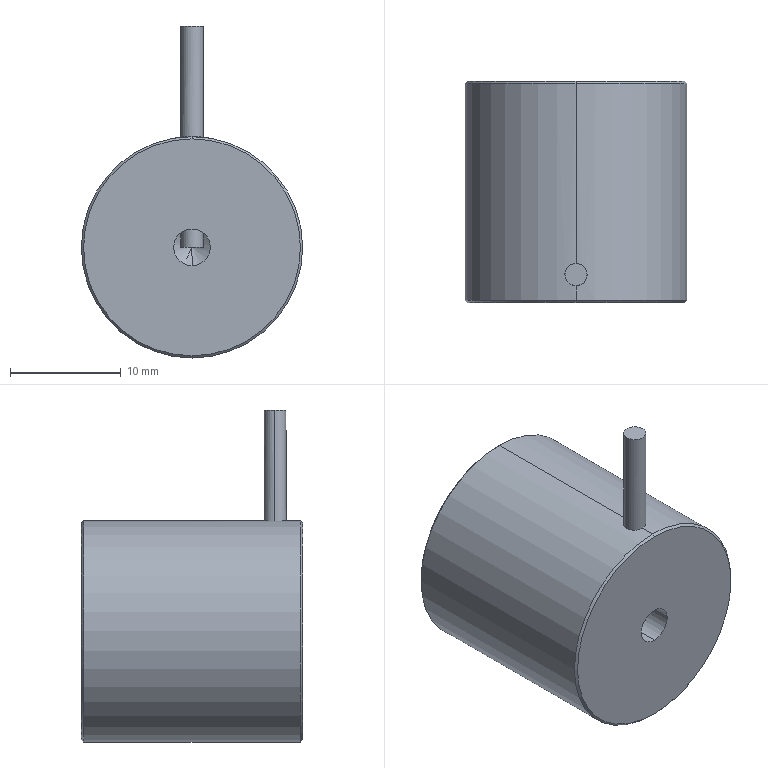Part | SolidWorks | features BaseBody 1 | 1 solid | 18 faces | box 20 x 20 x 30 mm | volume 6254 mm3 | cylinder 8 | cone 6 | plane 4 | commonest cylinder face diameters 2 x4 3.3 x2 20 x2
STEP:
#1=CARTESIAN_POINT('',(0.,20.,9.8));
#2=VERTEX_POINT('',#1);
#3=CARTESIAN_POINT('',(0.,19.8,10.));
#4=VERTEX_POINT('',#3);
#5=CARTESIAN_POINT('',(0.,20.,9.8));
#6=DIRECTION('',(0.,-0.7071,0.7071));
#7=VECTOR('',#6,1000.);
#8=LINE('',#5,#7);
#9=EDGE_CURVE('',#2,#4,#8,.T.);
#10=ORIENTED_EDGE('',*,*,#9,.F.);
#11=CARTESIAN_POINT('',(0.,20.,-9.8));
#12=VERTEX_POINT('',#11);
#13=CARTESIAN_POINT('',(0.,20.,0.));
#14=DIRECTION('',(0.,1.,0.));
#15=DIRECTION('',(0.,0.,1.));
#16=AXIS2_PLACEMENT_3D('',#13,#14,#15);
#17=CIRCLE('',#16,9.8);
#18=EDGE_CURVE('',#12,#2,#17,.T.);
#19=ORIENTED_EDGE('',*,*,#18,.F.);
#20=CARTESIAN_POINT('',(0.,19.8,-10.));
#21=VERTEX_POINT('',#20);
#22=CARTESIAN_POINT('',(0.,20.,-9.8));
#23=DIRECTION('',(0.,-0.7071,-0.7071));
#24=VECTOR('',#23,1000.);
#25=LINE('',#22,#24);
#26=EDGE_CURVE('',#12,#21,#25,.T.);
#27=ORIENTED_EDGE('',*,*,#26,.T.);
#28=CARTESIAN_POINT('',(0.,19.8,0.));
#29=DIRECTION('',(0.,-1.,0.));
#30=DIRECTION('',(0.,0.,1.));
#31=AXIS2_PLACEMENT_3D('',#28,#29,#30);
#32=CIRCLE('',#31,10.);
#33=EDGE_CURVE('',#4,#21,#32,.T.);
#34=ORIENTED_EDGE('',*,*,#33,.F.);
#35=EDGE_LOOP('',(#10,#19,#27,#34));
#36=FACE_OUTER_BOUND('',#35,.T.);
#37=CARTESIAN_POINT('',(0.,20.,0.));
#38=DIRECTION('',(0.,-1.,0.));
#39=DIRECTION('',(0.,0.,-1.));
#40=AXIS2_PLACEMENT_3D('',#37,#38,#39);
#41=CONICAL_SURFACE('',#40,9.8,0.7854);
#42=ADVANCED_FACE('',(#36),#41,.T.);
#43=CARTESIAN_POINT('',(0.,0.,-9.8));
#44=VERTEX_POINT('',#43);
#45=CARTESIAN_POINT('',(0.,0.2,-10.));
#46=VERTEX_POINT('',#45);
#47=CARTESIAN_POINT('',(0.,0.2,-10.));
#48=DIRECTION('',(0.,0.7071,-0.7071));
#49=VECTOR('',#48,1000.);
#50=LINE('',#47,#49);
#51=EDGE_CURVE('',#44,#46,#50,.T.);
#52=ORIENTED_EDGE('',*,*,#51,.F.);
#53=CARTESIAN_POINT('',(0.,0.,9.8));
#54=VERTEX_POINT('',#53);
#55=CARTESIAN_POINT('',(0.,0.,0.));
#56=DIRECTION('',(0.,-1.,0.));
#57=DIRECTION('',(0.,0.,1.));
#58=AXIS2_PLACEMENT_3D('',#55,#56,#57);
#59=CIRCLE('',#58,9.8);
#60=EDGE_CURVE('',#54,#44,#59,.T.);
#61=ORIENTED_EDGE('',*,*,#60,.F.);
#62=CARTESIAN_POINT('',(0.,0.2,10.));
#63=VERTEX_POINT('',#62);
#64=CARTESIAN_POINT('',(0.,0.2,10.));
#65=DIRECTION('',(0.,0.7071,0.7071));
#66=VECTOR('',#65,1000.);
#67=LINE('',#64,#66);
#68=EDGE_CURVE('',#54,#63,#67,.T.);
#69=ORIENTED_EDGE('',*,*,#68,.T.);
#70=CARTESIAN_POINT('',(0.,0.2,0.));
#71=DIRECTION('',(0.,1.,0.));
#72=DIRECTION('',(0.,0.,1.));
#73=AXIS2_PLACEMENT_3D('',#70,#71,#72);
#74=CIRCLE('',#73,10.);
#75=EDGE_CURVE('',#46,#63,#74,.T.);
#76=ORIENTED_EDGE('',*,*,#75,.F.);
#77=EDGE_LOOP('',(#52,#61,#69,#76));
#78=FACE_OUTER_BOUND('',#77,.T.);
#79=CARTESIAN_POINT('',(0.,0.2,0.));
#80=DIRECTION('',(0.,1.,0.));
#81=DIRECTION('',(0.,0.,1.));
#82=AXIS2_PLACEMENT_3D('',#79,#80,#81);
#83=CONICAL_SURFACE('',#82,10.,0.7854);
#84=ADVANCED_FACE('',(#78),#83,.T.);
#85=CARTESIAN_POINT('',(-1.,2.5,20.));
#86=VERTEX_POINT('',#85);
#87=CARTESIAN_POINT('',(1.,2.5,20.));
#88=VERTEX_POINT('',#87);
#89=CARTESIAN_POINT('',(0.,2.5,20.));
#90=DIRECTION('',(0.,0.,1.));
#91=DIRECTION('',(1.,0.,0.));
#92=AXIS2_PLACEMENT_3D('',#89,#90,#91);
#93=CIRCLE('',#92,1.);
#94=EDGE_CURVE('',#86,#88,#93,.T.);
#95=ORIENTED_EDGE('',*,*,#94,.T.);
#96=CARTESIAN_POINT('',(0.,2.5,20.));
#97=DIRECTION('',(0.,0.,1.));
#98=DIRECTION('',(1.,0.,0.));
#99=AXIS2_PLACEMENT_3D('',#96,#97,#98);
#100=CIRCLE('',#99,1.);
#101=EDGE_CURVE('',#88,#86,#100,.T.);
#102=ORIENTED_EDGE('',*,*,#101,.T.);
#103=EDGE_LOOP('',(#95,#102));
#104=FACE_OUTER_BOUND('',#103,.T.);
#105=CARTESIAN_POINT('',(0.,2.5,20.));
#106=DIRECTION('',(0.,0.,1.));
#107=DIRECTION('',(1.,0.,0.));
#108=AXIS2_PLACEMENT_3D('',#105,#106,#107);
#109=PLANE('',#108);
#110=ADVANCED_FACE('',(#104),#109,.T.);
#111=CARTESIAN_POINT('',(1.,2.5,9.95));
#112=VERTEX_POINT('',#111);
#113=CARTESIAN_POINT('',(1.,2.5,20.));
#114=DIRECTION('',(0.,0.,-1.));
#115=VECTOR('',#114,1000.);
#116=LINE('',#113,#115);
#117=EDGE_CURVE('',#88,#112,#116,.T.);
#118=ORIENTED_EDGE('',*,*,#117,.F.);
#119=ORIENTED_EDGE('',*,*,#94,.F.);
#120=CARTESIAN_POINT('',(-1.,2.5,9.95));
#121=VERTEX_POINT('',#120);
#122=CARTESIAN_POINT('',(-1.,2.5,20.));
#123=DIRECTION('',(0.,0.,-1.));
#124=VECTOR('',#123,1000.);
#125=LINE('',#122,#124);
#126=EDGE_CURVE('',#86,#121,#125,.T.);
#127=ORIENTED_EDGE('',*,*,#126,.T.);
#128=CARTESIAN_POINT('',(0.,1.5,10.));
#129=VERTEX_POINT('',#128);
#130=CARTESIAN_POINT('',(-1.,2.5,9.95));
#131=CARTESIAN_POINT('',(-1.,2.438,9.95));
#132=CARTESIAN_POINT('',(-0.9942,2.374,9.95));
#133=CARTESIAN_POINT('',(-0.9756,2.278,9.952));
#134=CARTESIAN_POINT('',(-0.9677,2.246,9.953));
#135=CARTESIAN_POINT('',(-0.9532,2.197,9.954));
#136=CARTESIAN_POINT('',(-0.9453,2.173,9.955));
#137=CARTESIAN_POINT('',(-0.9349,2.145,9.956));
#138=CARTESIAN_POINT('',(-0.9302,2.133,9.957));
#139=CARTESIAN_POINT('',(-0.927,2.125,9.957));
#140=CARTESIAN_POINT('',(-0.9247,2.119,9.957));
#141=CARTESIAN_POINT('',(-0.9067,2.076,9.959));
#142=CARTESIAN_POINT('',(-0.883,2.026,9.961));
#143=CARTESIAN_POINT('',(-0.8138,1.915,9.967));
#144=CARTESIAN_POINT('',(-0.7677,1.853,9.971));
#145=CARTESIAN_POINT('',(-0.646,1.732,9.979));
#146=CARTESIAN_POINT('',(-0.5848,1.686,9.983));
#147=CARTESIAN_POINT('',(-0.5016,1.634,9.987));
#148=CARTESIAN_POINT('',(-0.4752,1.62,9.989));
#149=CARTESIAN_POINT('',(-0.4384,1.601,9.99));
#150=CARTESIAN_POINT('',(-0.4206,1.593,9.991));
#151=CARTESIAN_POINT('',(-0.4012,1.584,9.992));
#152=CARTESIAN_POINT('',(-0.3931,1.581,9.992));
#153=CARTESIAN_POINT('',(-0.3878,1.578,9.992));
#154=CARTESIAN_POINT('',(-0.3866,1.578,9.993));
#155=CARTESIAN_POINT('',(-0.2552,1.523,9.998));
#156=CARTESIAN_POINT('',(-0.1238,1.5,10.));
#157=CARTESIAN_POINT('',(0.,1.5,10.));
#158=B_SPLINE_CURVE_WITH_KNOTS('',3,(#130,#131,#132,#133,#134,#135,#136,#137,#138,#139,#140,#141,#142,#143,#144,#145,#146,#147,#148,#149,#150,#151,#152,#153,#154,#155,#156,#157),.UNSPECIFIED.,.F.,.F.,(4,2,2,1,1,2,2,2,2,2,2,1,1,2,2,4),(0.,0.125,0.1875,0.2188,0.2344,0.2422,0.25,0.375,0.5,0.625,0.6875,0.7188,0.7344,0.7422,0.75,1.),.UNSPECIFIED.);
#159=EDGE_CURVE('',#121,#129,#158,.T.);
#160=ORIENTED_EDGE('',*,*,#159,.T.);
#161=CARTESIAN_POINT('',(0.,1.5,10.));
#162=CARTESIAN_POINT('',(0.06188,1.5,10.));
#163=CARTESIAN_POINT('',(0.1256,1.506,9.999));
#164=CARTESIAN_POINT('',(0.222,1.524,9.998));
#165=CARTESIAN_POINT('',(0.2542,1.532,9.997));
#166=CARTESIAN_POINT('',(0.3025,1.547,9.995));
#167=CARTESIAN_POINT('',(0.3267,1.555,9.995));
#168=CARTESIAN_POINT('',(0.3547,1.565,9.994));
#169=CARTESIAN_POINT('',(0.3667,1.57,9.993));
#170=CARTESIAN_POINT('',(0.3747,1.573,9.993));
#171=CARTESIAN_POINT('',(0.3801,1.575,9.993));
#172=CARTESIAN_POINT('',(0.4653,1.61,9.99));
#173=CARTESIAN_POINT('',(0.5848,1.671,9.984));
#174=CARTESIAN_POINT('',(0.7683,1.854,9.971));
#175=CARTESIAN_POINT('',(0.814,1.915,9.967));
#176=CARTESIAN_POINT('',(0.8659,1.999,9.963));
#177=CARTESIAN_POINT('',(0.8805,2.025,9.961));
#178=CARTESIAN_POINT('',(0.899,2.062,9.96));
#179=CARTESIAN_POINT('',(0.9075,2.08,9.959));
#180=CARTESIAN_POINT('',(0.9161,2.099,9.958));
#181=CARTESIAN_POINT('',(0.9195,2.107,9.958));
#182=CARTESIAN_POINT('',(0.9217,2.112,9.957));
#183=CARTESIAN_POINT('',(0.9222,2.113,9.957));
#184=CARTESIAN_POINT('',(0.9767,2.245,9.952));
#185=CARTESIAN_POINT('',(1.,2.376,9.95));
#186=CARTESIAN_POINT('',(1.,2.5,9.95));
#187=B_SPLINE_CURVE_WITH_KNOTS('',3,(#161,#162,#163,#164,#165,#166,#167,#168,#169,#170,#171,#172,#173,#174,#175,#176,#177,#178,#179,#180,#181,#182,#183,#184,#185,#186),.UNSPECIFIED.,.F.,.F.,(4,2,2,1,1,2,2,2,2,2,1,1,2,2,4),(0.,0.125,0.1875,0.2187,0.2344,0.2422,0.25,0.5,0.625,0.6875,0.7188,0.7344,0.7422,0.75,1.),.UNSPECIFIED.);
#188=EDGE_CURVE('',#129,#112,#187,.T.);
#189=ORIENTED_EDGE('',*,*,#188,.T.);
#190=EDGE_LOOP('',(#118,#119,#127,#160,#189));
#191=FACE_OUTER_BOUND('',#190,.T.);
#192=CARTESIAN_POINT('',(0.,2.5,20.));
#193=DIRECTION('',(0.,0.,-1.));
#194=DIRECTION('',(-1.,0.,0.));
#195=AXIS2_PLACEMENT_3D('',#192,#193,#194);
#196=CYLINDRICAL_SURFACE('',#195,1.);
#197=ADVANCED_FACE('',(#191),#196,.T.);
#198=CARTESIAN_POINT('',(1.,2.5,1.312));
#199=VERTEX_POINT('',#198);
#200=CARTESIAN_POINT('',(1.,2.5,0.));
#201=VERTEX_POINT('',#200);
#202=CARTESIAN_POINT('',(1.,2.5,20.));
#203=DIRECTION('',(0.,0.,-1.));
#204=VECTOR('',#203,1000.);
#205=LINE('',#202,#204);
#206=EDGE_CURVE('',#199,#201,#205,.T.);
#207=ORIENTED_EDGE('',*,*,#206,.F.);
#208=CARTESIAN_POINT('',(0.,1.5,1.65));
#209=VERTEX_POINT('',#208);
#210=CARTESIAN_POINT('',(1.,2.5,1.312));
#211=CARTESIAN_POINT('',(1.,2.439,1.312));
#212=CARTESIAN_POINT('',(0.9944,2.375,1.317));
#213=CARTESIAN_POINT('',(0.9754,2.277,1.331));
#214=CARTESIAN_POINT('',(0.9673,2.244,1.337));
#215=CARTESIAN_POINT('',(0.9523,2.194,1.348));
#216=CARTESIAN_POINT('',(0.944,2.169,1.353));
#217=CARTESIAN_POINT('',(0.9347,2.145,1.36));
#218=CARTESIAN_POINT('',(0.9283,2.128,1.364));
#219=CARTESIAN_POINT('',(0.9241,2.118,1.367));
#220=CARTESIAN_POINT('',(0.9105,2.086,1.376));
#221=CARTESIAN_POINT('',(0.8978,2.058,1.385));
#222=CARTESIAN_POINT('',(0.875,2.016,1.399));
#223=CARTESIAN_POINT('',(0.8628,1.994,1.407));
#224=CARTESIAN_POINT('',(0.8467,1.968,1.416));
#225=CARTESIAN_POINT('',(0.8383,1.955,1.421));
#226=CARTESIAN_POINT('',(0.8345,1.949,1.423));
#227=CARTESIAN_POINT('',(0.832,1.945,1.425));
#228=CARTESIAN_POINT('',(0.8297,1.942,1.426));
#229=CARTESIAN_POINT('',(0.8265,1.937,1.428));
#230=CARTESIAN_POINT('',(0.8162,1.921,1.434));
#231=CARTESIAN_POINT('',(0.7872,1.883,1.45));
#232=CARTESIAN_POINT('',(0.7753,1.868,1.457));
#233=CARTESIAN_POINT('',(0.7533,1.842,1.468));
#234=CARTESIAN_POINT('',(0.7412,1.829,1.474));
#235=CARTESIAN_POINT('',(0.7252,1.811,1.482));
#236=CARTESIAN_POINT('',(0.7179,1.804,1.486));
#237=CARTESIAN_POINT('',(0.713,1.799,1.488));
#238=CARTESIAN_POINT('',(0.7096,1.795,1.49));
#239=CARTESIAN_POINT('',(0.6521,1.738,1.517));
#240=CARTESIAN_POINT('',(0.5949,1.694,1.54));
#241=CARTESIAN_POINT('',(0.5136,1.641,1.568));
#242=CARTESIAN_POINT('',(0.4872,1.626,1.576));
#243=CARTESIAN_POINT('',(0.4492,1.606,1.588));
#244=CARTESIAN_POINT('',(0.4306,1.597,1.593));
#245=CARTESIAN_POINT('',(0.4097,1.588,1.598));
#246=CARTESIAN_POINT('',(0.4009,1.584,1.601));
#247=CARTESIAN_POINT('',(0.395,1.581,1.602));
#248=CARTESIAN_POINT('',(0.3933,1.581,1.602));
#249=CARTESIAN_POINT('',(0.2614,1.525,1.634));
#250=CARTESIAN_POINT('',(0.1277,1.5,1.65));
#251=CARTESIAN_POINT('',(0.,1.5,1.65));
#252=B_SPLINE_CURVE_WITH_KNOTS('',3,(#210,#211,#212,#213,#214,#215,#216,#217,#218,#219,#220,#221,#222,#223,#224,#225,#226,#227,#228,#229,#230,#231,#232,#233,#234,#235,#236,#237,#238,#239,#240,#241,#242,#243,#244,#245,#246,#247,#248,#249,#250,#251),.UNSPECIFIED.,.F.,.F.,(4,2,2,1,2,2,2,1,1,1,2,2,2,2,1,1,2,2,2,2,1,1,2,2,4),(0.,0.125,0.1875,0.2188,0.2344,0.25,0.3125,0.3438,0.3594,0.3672,0.3711,0.375,0.4375,0.4688,0.4844,0.4922,0.4961,0.5,0.625,0.6875,0.7188,0.7344,0.7422,0.75,1.),.UNSPECIFIED.);
#253=EDGE_CURVE('',#199,#209,#252,.T.);
#254=ORIENTED_EDGE('',*,*,#253,.T.);
#255=CARTESIAN_POINT('',(-1.,2.5,1.312));
#256=VERTEX_POINT('',#255);
#257=CARTESIAN_POINT('',(0.,1.5,1.65));
#258=CARTESIAN_POINT('',(-0.06387,1.5,1.65));
#259=CARTESIAN_POINT('',(-0.1292,1.506,1.646));
#260=CARTESIAN_POINT('',(-0.2272,1.526,1.634));
#261=CARTESIAN_POINT('',(-0.26,1.534,1.63));
#262=CARTESIAN_POINT('',(-0.3088,1.549,1.621));
#263=CARTESIAN_POINT('',(-0.3331,1.557,1.616));
#264=CARTESIAN_POINT('',(-0.3613,1.567,1.61));
#265=CARTESIAN_POINT('',(-0.3734,1.572,1.607));
#266=CARTESIAN_POINT('',(-0.3814,1.576,1.605));
#267=CARTESIAN_POINT('',(-0.3865,1.578,1.604));
#268=CARTESIAN_POINT('',(-0.4353,1.598,1.592));
#269=CARTESIAN_POINT('',(-0.4867,1.624,1.577));
#270=CARTESIAN_POINT('',(-0.5681,1.676,1.549));
#271=CARTESIAN_POINT('',(-0.5959,1.696,1.539));
#272=CARTESIAN_POINT('',(-0.638,1.73,1.522));
#273=CARTESIAN_POINT('',(-0.6592,1.748,1.513));
#274=CARTESIAN_POINT('',(-0.6838,1.77,1.502));
#275=CARTESIAN_POINT('',(-0.6961,1.782,1.496));
#276=CARTESIAN_POINT('',(-0.7013,1.787,1.494));
#277=CARTESIAN_POINT('',(-0.7048,1.791,1.492));
#278=CARTESIAN_POINT('',(-0.7058,1.792,1.491));
#279=CARTESIAN_POINT('',(-0.7495,1.835,1.471));
#280=CARTESIAN_POINT('',(-0.7778,1.871,1.456));
#281=CARTESIAN_POINT('',(-0.8067,1.909,1.44));
#282=CARTESIAN_POINT('',(-0.814,1.919,1.435));
#283=CARTESIAN_POINT('',(-0.822,1.93,1.431));
#284=CARTESIAN_POINT('',(-0.8252,1.935,1.429));
#285=CARTESIAN_POINT('',(-0.8277,1.939,1.427));
#286=CARTESIAN_POINT('',(-0.8286,1.94,1.427));
#287=CARTESIAN_POINT('',(-0.829,1.941,1.427));
#288=CARTESIAN_POINT('',(-0.8282,1.94,1.427));
#289=CARTESIAN_POINT('',(-0.8497,1.972,1.415));
#290=CARTESIAN_POINT('',(-0.8672,2.001,1.404));
#291=CARTESIAN_POINT('',(-0.8899,2.044,1.389));
#292=CARTESIAN_POINT('',(-0.9004,2.065,1.383));
#293=CARTESIAN_POINT('',(-0.9097,2.085,1.377));
#294=CARTESIAN_POINT('',(-0.9156,2.098,1.373));
#295=CARTESIAN_POINT('',(-0.9177,2.103,1.371));
#296=CARTESIAN_POINT('',(-0.9771,2.243,1.331));
#297=CARTESIAN_POINT('',(-1.,2.377,1.312));
#298=CARTESIAN_POINT('',(-1.,2.5,1.312));
#299=B_SPLINE_CURVE_WITH_KNOTS('',3,(#257,#258,#259,#260,#261,#262,#263,#264,#265,#266,#267,#268,#269,#270,#271,#272,#273,#274,#275,#276,#277,#278,#279,#280,#281,#282,#283,#284,#285,#286,#287,#288,#289,#290,#291,#292,#293,#294,#295,#296,#297,#298),.UNSPECIFIED.,.F.,.F.,(4,2,2,1,1,2,2,2,2,1,1,1,2,2,2,2,1,1,2,2,2,1,2,2,4),(0.,0.125,0.1875,0.2188,0.2344,0.2422,0.25,0.375,0.4375,0.4688,0.4844,0.4922,0.4961,0.5,0.5625,0.5938,0.6094,0.6172,0.6211,0.625,0.6875,0.7188,0.7344,0.75,1.),.UNSPECIFIED.);
#300=EDGE_CURVE('',#209,#256,#299,.T.);
#301=ORIENTED_EDGE('',*,*,#300,.T.);
#302=CARTESIAN_POINT('',(-1.,2.5,0.));
#303=VERTEX_POINT('',#302);
#304=CARTESIAN_POINT('',(-1.,2.5,20.));
#305=DIRECTION('',(0.,0.,-1.));
#306=VECTOR('',#305,1000.);
#307=LINE('',#304,#306);
#308=EDGE_CURVE('',#256,#303,#307,.T.);
#309=ORIENTED_EDGE('',*,*,#308,.T.);
#310=CARTESIAN_POINT('',(0.,2.5,0.));
#311=DIRECTION('',(0.,0.,1.));
#312=DIRECTION('',(1.,0.,0.));
#313=AXIS2_PLACEMENT_3D('',#310,#311,#312);
#314=CIRCLE('',#313,1.);
#315=EDGE_CURVE('',#303,#201,#314,.T.);
#316=ORIENTED_EDGE('',*,*,#315,.T.);
#317=EDGE_LOOP('',(#207,#254,#301,#309,#316));
#318=FACE_OUTER_BOUND('',#317,.T.);
#319=CARTESIAN_POINT('',(0.,2.5,20.));
#320=DIRECTION('',(0.,0.,-1.));
#321=DIRECTION('',(-1.,0.,0.));
#322=AXIS2_PLACEMENT_3D('',#319,#320,#321);
#323=CYLINDRICAL_SURFACE('',#322,1.);
#324=ADVANCED_FACE('',(#318),#323,.T.);
#325=ORIENTED_EDGE('',*,*,#315,.F.);
#326=CARTESIAN_POINT('',(0.,2.5,0.));
#327=DIRECTION('',(0.,0.,1.));
#328=DIRECTION('',(1.,0.,0.));
#329=AXIS2_PLACEMENT_3D('',#326,#327,#328);
#330=CIRCLE('',#329,1.);
#331=EDGE_CURVE('',#201,#303,#330,.T.);
#332=ORIENTED_EDGE('',*,*,#331,.F.);
#333=EDGE_LOOP('',(#325,#332));
#334=FACE_OUTER_BOUND('',#333,.T.);
#335=CARTESIAN_POINT('',(0.,2.5,0.));
#336=DIRECTION('',(0.,0.,1.));
#337=DIRECTION('',(1.,0.,0.));
#338=AXIS2_PLACEMENT_3D('',#335,#336,#337);
#339=PLANE('',#338);
#340=ADVANCED_FACE('',(#334),#339,.F.);
#341=CARTESIAN_POINT('',(0.,8.091,0.));
#342=VERTEX_POINT('',#341);
#343=CARTESIAN_POINT('',(0.,7.1,1.65));
#344=VERTEX_POINT('',#343);
#345=CARTESIAN_POINT('',(0.,7.1,1.65));
#346=DIRECTION('',(0.,-0.515,0.8572));
#347=VECTOR('',#346,1000.);
#348=LINE('',#345,#347);
#349=EDGE_CURVE('',#342,#344,#348,.T.);
#350=ORIENTED_EDGE('',*,*,#349,.F.);
#351=CARTESIAN_POINT('',(0.,7.1,-1.65));
#352=VERTEX_POINT('',#351);
#353=CARTESIAN_POINT('',(0.,7.1,-1.65));
#354=DIRECTION('',(0.,-0.515,-0.8572));
#355=VECTOR('',#354,1000.);
#356=LINE('',#353,#355);
#357=EDGE_CURVE('',#342,#352,#356,.T.);
#358=ORIENTED_EDGE('',*,*,#357,.T.);
#359=CARTESIAN_POINT('',(0.,7.1,0.));
#360=DIRECTION('',(0.,-1.,0.));
#361=DIRECTION('',(0.,0.,-1.));
#362=AXIS2_PLACEMENT_3D('',#359,#360,#361);
#363=CIRCLE('',#362,1.65);
#364=EDGE_CURVE('',#352,#344,#363,.T.);
#365=ORIENTED_EDGE('',*,*,#364,.T.);
#366=EDGE_LOOP('',(#350,#358,#365));
#367=FACE_OUTER_BOUND('',#366,.T.);
#368=CARTESIAN_POINT('',(0.,7.1,0.));
#369=DIRECTION('',(0.,-1.,0.));
#370=DIRECTION('',(0.,0.,-1.));
#371=AXIS2_PLACEMENT_3D('',#368,#369,#370);
#372=CONICAL_SURFACE('',#371,1.65,1.03);
#373=ADVANCED_FACE('',(#367),#372,.F.);
#374=CARTESIAN_POINT('',(0.,0.,-1.65));
#375=VERTEX_POINT('',#374);
#376=CARTESIAN_POINT('',(0.,0.,1.65));
#377=VERTEX_POINT('',#376);
#378=CARTESIAN_POINT('',(0.,0.,0.));
#379=DIRECTION('',(0.,-1.,0.));
#380=DIRECTION('',(0.,0.,-1.));
#381=AXIS2_PLACEMENT_3D('',#378,#379,#380);
#382=CIRCLE('',#381,1.65);
#383=EDGE_CURVE('',#375,#377,#382,.T.);
#384=ORIENTED_EDGE('',*,*,#383,.F.);
#385=CARTESIAN_POINT('',(0.,0.,0.));
#386=DIRECTION('',(0.,-1.,0.));
#387=DIRECTION('',(0.,0.,-1.));
#388=AXIS2_PLACEMENT_3D('',#385,#386,#387);
#389=CIRCLE('',#388,1.65);
#390=EDGE_CURVE('',#377,#375,#389,.T.);
#391=ORIENTED_EDGE('',*,*,#390,.F.);
#392=EDGE_LOOP('',(#384,#391));
#393=FACE_BOUND('',#392,.T.);
#394=ORIENTED_EDGE('',*,*,#60,.T.);
#395=CARTESIAN_POINT('',(0.,0.,0.));
#396=DIRECTION('',(0.,-1.,0.));
#397=DIRECTION('',(0.,0.,1.));
#398=AXIS2_PLACEMENT_3D('',#395,#396,#397);
#399=CIRCLE('',#398,9.8);
#400=EDGE_CURVE('',#44,#54,#399,.T.);
#401=ORIENTED_EDGE('',*,*,#400,.T.);
#402=EDGE_LOOP('',(#394,#401));
#403=FACE_OUTER_BOUND('',#402,.T.);
#404=CARTESIAN_POINT('',(0.,0.,0.));
#405=DIRECTION('',(0.,1.,0.));
#406=DIRECTION('',(1.,0.,0.));
#407=AXIS2_PLACEMENT_3D('',#404,#405,#406);
#408=PLANE('',#407);
#409=ADVANCED_FACE('',(#393,#403),#408,.F.);
#410=ORIENTED_EDGE('',*,*,#18,.T.);
#411=CARTESIAN_POINT('',(0.,20.,0.));
#412=DIRECTION('',(0.,1.,0.));
#413=DIRECTION('',(0.,0.,1.));
#414=AXIS2_PLACEMENT_3D('',#411,#412,#413);
#415=CIRCLE('',#414,9.8);
#416=EDGE_CURVE('',#2,#12,#415,.T.);
#417=ORIENTED_EDGE('',*,*,#416,.T.);
#418=EDGE_LOOP('',(#410,#417));
#419=FACE_OUTER_BOUND('',#418,.T.);
#420=CARTESIAN_POINT('',(0.,20.,0.));
#421=DIRECTION('',(0.,1.,0.));
#422=DIRECTION('',(1.,0.,0.));
#423=AXIS2_PLACEMENT_3D('',#420,#421,#422);
#424=PLANE('',#423);
#425=ADVANCED_FACE('',(#419),#424,.T.);
#426=CARTESIAN_POINT('',(0.,3.5,1.65));
#427=VERTEX_POINT('',#426);
#428=CARTESIAN_POINT('',(0.,0.,1.65));
#429=DIRECTION('',(0.,-1.,0.));
#430=VECTOR('',#429,1000.);
#431=LINE('',#428,#430);
#432=EDGE_CURVE('',#344,#427,#431,.T.);
#433=ORIENTED_EDGE('',*,*,#432,.F.);
#434=ORIENTED_EDGE('',*,*,#364,.F.);
#435=CARTESIAN_POINT('',(0.,0.,-1.65));
#436=DIRECTION('',(0.,-1.,0.));
#437=VECTOR('',#436,1000.);
#438=LINE('',#435,#437);
#439=EDGE_CURVE('',#352,#375,#438,.T.);
#440=ORIENTED_EDGE('',*,*,#439,.T.);
#441=ORIENTED_EDGE('',*,*,#383,.T.);
#442=CARTESIAN_POINT('',(0.,0.,1.65));
#443=DIRECTION('',(0.,-1.,0.));
#444=VECTOR('',#443,1000.);
#445=LINE('',#442,#444);
#446=EDGE_CURVE('',#209,#377,#445,.T.);
#447=ORIENTED_EDGE('',*,*,#446,.F.);
#448=ORIENTED_EDGE('',*,*,#253,.F.);
#449=CARTESIAN_POINT('',(0.,3.5,1.65));
#450=CARTESIAN_POINT('',(0.06396,3.5,1.65));
#451=CARTESIAN_POINT('',(0.1293,3.494,1.646));
#452=CARTESIAN_POINT('',(0.2276,3.474,1.634));
#453=CARTESIAN_POINT('',(0.2603,3.466,1.63));
#454=CARTESIAN_POINT('',(0.3092,3.451,1.621));
#455=CARTESIAN_POINT('',(0.3336,3.443,1.616));
#456=CARTESIAN_POINT('',(0.3619,3.432,1.61));
#457=CARTESIAN_POINT('',(0.3739,3.427,1.607));
#458=CARTESIAN_POINT('',(0.382,3.424,1.605));
#459=CARTESIAN_POINT('',(0.3871,3.422,1.604));
#460=CARTESIAN_POINT('',(0.4358,3.401,1.592));
#461=CARTESIAN_POINT('',(0.4871,3.376,1.577));
#462=CARTESIAN_POINT('',(0.5685,3.323,1.549));
#463=CARTESIAN_POINT('',(0.5964,3.304,1.538));
#464=CARTESIAN_POINT('',(0.6385,3.27,1.521));
#465=CARTESIAN_POINT('',(0.6596,3.252,1.512));
#466=CARTESIAN_POINT('',(0.6843,3.229,1.501));
#467=CARTESIAN_POINT('',(0.6966,3.218,1.496));
#468=CARTESIAN_POINT('',(0.7018,3.212,1.493));
#469=CARTESIAN_POINT('',(0.7053,3.209,1.492));
#470=CARTESIAN_POINT('',(0.7063,3.208,1.491));
#471=CARTESIAN_POINT('',(0.7493,3.165,1.471));
#472=CARTESIAN_POINT('',(0.7774,3.13,1.456));
#473=CARTESIAN_POINT('',(0.8062,3.092,1.44));
#474=CARTESIAN_POINT('',(0.8137,3.081,1.436));
#475=CARTESIAN_POINT('',(0.8219,3.07,1.431));
#476=CARTESIAN_POINT('',(0.8252,3.065,1.429));
#477=CARTESIAN_POINT('',(0.828,3.061,1.427));
#478=CARTESIAN_POINT('',(0.8289,3.059,1.427));
#479=CARTESIAN_POINT('',(0.8294,3.059,1.426));
#480=CARTESIAN_POINT('',(0.8286,3.06,1.427));
#481=CARTESIAN_POINT('',(0.8502,3.028,1.414));
#482=CARTESIAN_POINT('',(0.8677,2.998,1.404));
#483=CARTESIAN_POINT('',(0.8903,2.956,1.389));
#484=CARTESIAN_POINT('',(0.9008,2.935,1.382));
#485=CARTESIAN_POINT('',(0.91,2.915,1.376));
#486=CARTESIAN_POINT('',(0.9159,2.901,1.372));
#487=CARTESIAN_POINT('',(0.9179,2.897,1.371));
#488=CARTESIAN_POINT('',(0.9772,2.756,1.331));
#489=CARTESIAN_POINT('',(1.,2.623,1.312));
#490=CARTESIAN_POINT('',(1.,2.5,1.312));
#491=B_SPLINE_CURVE_WITH_KNOTS('',3,(#449,#450,#451,#452,#453,#454,#455,#456,#457,#458,#459,#460,#461,#462,#463,#464,#465,#466,#467,#468,#469,#470,#471,#472,#473,#474,#475,#476,#477,#478,#479,#480,#481,#482,#483,#484,#485,#486,#487,#488,#489,#490),.UNSPECIFIED.,.F.,.F.,(4,2,2,1,1,2,2,2,2,1,1,1,2,2,2,2,1,1,2,2,2,1,2,2,4),(0.,0.125,0.1875,0.2188,0.2344,0.2422,0.25,0.375,0.4375,0.4688,0.4844,0.4922,0.4961,0.5,0.5625,0.5938,0.6094,0.6172,0.6211,0.625,0.6875,0.7188,0.7344,0.75,1.),.UNSPECIFIED.);
#492=EDGE_CURVE('',#427,#199,#491,.T.);
#493=ORIENTED_EDGE('',*,*,#492,.F.);
#494=EDGE_LOOP('',(#433,#434,#440,#441,#447,#448,#493));
#495=FACE_OUTER_BOUND('',#494,.T.);
#496=CARTESIAN_POINT('',(0.,0.,0.));
#497=DIRECTION('',(0.,-1.,0.));
#498=DIRECTION('',(0.,0.,-1.));
#499=AXIS2_PLACEMENT_3D('',#496,#497,#498);
#500=CYLINDRICAL_SURFACE('',#499,1.65);
#501=ADVANCED_FACE('',(#495),#500,.F.);
#502=CARTESIAN_POINT('',(0.,3.5,10.));
#503=VERTEX_POINT('',#502);
#504=CARTESIAN_POINT('',(0.,20.,10.));
#505=DIRECTION('',(0.,-1.,0.));
#506=VECTOR('',#505,1000.);
#507=LINE('',#504,#506);
#508=EDGE_CURVE('',#4,#503,#507,.T.);
#509=ORIENTED_EDGE('',*,*,#508,.F.);
#510=ORIENTED_EDGE('',*,*,#33,.T.);
#511=CARTESIAN_POINT('',(0.,20.,-10.));
#512=DIRECTION('',(0.,-1.,0.));
#513=VECTOR('',#512,1000.);
#514=LINE('',#511,#513);
#515=EDGE_CURVE('',#21,#46,#514,.T.);
#516=ORIENTED_EDGE('',*,*,#515,.T.);
#517=ORIENTED_EDGE('',*,*,#75,.T.);
#518=CARTESIAN_POINT('',(0.,20.,10.));
#519=DIRECTION('',(0.,-1.,0.));
#520=VECTOR('',#519,1000.);
#521=LINE('',#518,#520);
#522=EDGE_CURVE('',#129,#63,#521,.T.);
#523=ORIENTED_EDGE('',*,*,#522,.F.);
#524=ORIENTED_EDGE('',*,*,#159,.F.);
#525=CARTESIAN_POINT('',(0.,3.5,10.));
#526=CARTESIAN_POINT('',(-0.09534,3.5,10.));
#527=CARTESIAN_POINT('',(-0.2094,3.487,9.998));
#528=CARTESIAN_POINT('',(-0.4562,3.399,9.99));
#529=CARTESIAN_POINT('',(-0.5888,3.325,9.983));
#530=CARTESIAN_POINT('',(-0.825,3.089,9.967));
#531=CARTESIAN_POINT('',(-0.8996,2.956,9.96));
#532=CARTESIAN_POINT('',(-0.9867,2.709,9.952));
#533=CARTESIAN_POINT('',(-1.,2.595,9.95));
#534=CARTESIAN_POINT('',(-1.,2.5,9.95));
#535=B_SPLINE_CURVE_WITH_KNOTS('',3,(#525,#526,#527,#528,#529,#530,#531,#532,#533,#534),.UNSPECIFIED.,.F.,.F.,(4,2,2,2,4),(0.,0.25,0.5,0.75,1.),.UNSPECIFIED.);
#536=EDGE_CURVE('',#503,#121,#535,.T.);
#537=ORIENTED_EDGE('',*,*,#536,.F.);
#538=EDGE_LOOP('',(#509,#510,#516,#517,#523,#524,#537));
#539=FACE_OUTER_BOUND('',#538,.T.);
#540=CARTESIAN_POINT('',(0.,20.,0.));
#541=DIRECTION('',(0.,-1.,0.));
#542=DIRECTION('',(0.,0.,-1.));
#543=AXIS2_PLACEMENT_3D('',#540,#541,#542);
#544=CYLINDRICAL_SURFACE('',#543,10.);
#545=ADVANCED_FACE('',(#539),#544,.T.);
#546=CARTESIAN_POINT('',(0.,19.8,0.));
#547=DIRECTION('',(0.,-1.,0.));
#548=DIRECTION('',(0.,0.,1.));
#549=AXIS2_PLACEMENT_3D('',#546,#547,#548);
#550=CIRCLE('',#549,10.);
#551=EDGE_CURVE('',#21,#4,#550,.T.);
#552=ORIENTED_EDGE('',*,*,#551,.T.);
#553=ORIENTED_EDGE('',*,*,#508,.T.);
#554=CARTESIAN_POINT('',(1.,2.5,9.95));
#555=CARTESIAN_POINT('',(1.,2.562,9.95));
#556=CARTESIAN_POINT('',(0.9942,2.626,9.95));
#557=CARTESIAN_POINT('',(0.9756,2.722,9.952));
#558=CARTESIAN_POINT('',(0.9677,2.754,9.953));
#559=CARTESIAN_POINT('',(0.9533,2.802,9.954));
#560=CARTESIAN_POINT('',(0.9454,2.827,9.955));
#561=CARTESIAN_POINT('',(0.935,2.855,9.956));
#562=CARTESIAN_POINT('',(0.9303,2.867,9.957));
#563=CARTESIAN_POINT('',(0.9272,2.875,9.957));
#564=CARTESIAN_POINT('',(0.9249,2.88,9.957));
#565=CARTESIAN_POINT('',(0.8899,2.965,9.96));
#566=CARTESIAN_POINT('',(0.8292,3.085,9.966));
#567=CARTESIAN_POINT('',(0.6464,3.268,9.979));
#568=CARTESIAN_POINT('',(0.5852,3.313,9.983));
#569=CARTESIAN_POINT('',(0.502,3.365,9.987));
#570=CARTESIAN_POINT('',(0.4756,3.38,9.989));
#571=CARTESIAN_POINT('',(0.4388,3.399,9.99));
#572=CARTESIAN_POINT('',(0.421,3.407,9.991));
#573=CARTESIAN_POINT('',(0.4016,3.416,9.992));
#574=CARTESIAN_POINT('',(0.3936,3.419,9.992));
#575=CARTESIAN_POINT('',(0.3883,3.422,9.992));
#576=CARTESIAN_POINT('',(0.3871,3.422,9.993));
#577=CARTESIAN_POINT('',(0.2555,3.477,9.998));
#578=CARTESIAN_POINT('',(0.1239,3.5,10.));
#579=CARTESIAN_POINT('',(0.,3.5,10.));
#580=B_SPLINE_CURVE_WITH_KNOTS('',3,(#554,#555,#556,#557,#558,#559,#560,#561,#562,#563,#564,#565,#566,#567,#568,#569,#570,#571,#572,#573,#574,#575,#576,#577,#578,#579),.UNSPECIFIED.,.F.,.F.,(4,2,2,1,1,2,2,2,2,2,1,1,2,2,4),(0.,0.125,0.1875,0.2188,0.2344,0.2422,0.25,0.5,0.625,0.6875,0.7188,0.7344,0.7422,0.75,1.),.UNSPECIFIED.);
#581=EDGE_CURVE('',#112,#503,#580,.T.);
#582=ORIENTED_EDGE('',*,*,#581,.F.);
#583=ORIENTED_EDGE('',*,*,#188,.F.);
#584=ORIENTED_EDGE('',*,*,#522,.T.);
#585=CARTESIAN_POINT('',(0.,0.2,0.));
#586=DIRECTION('',(0.,1.,0.));
#587=DIRECTION('',(0.,0.,1.));
#588=AXIS2_PLACEMENT_3D('',#585,#586,#587);
#589=CIRCLE('',#588,10.);
#590=EDGE_CURVE('',#63,#46,#589,.T.);
#591=ORIENTED_EDGE('',*,*,#590,.T.);
#592=ORIENTED_EDGE('',*,*,#515,.F.);
#593=EDGE_LOOP('',(#552,#553,#582,#583,#584,#591,#592));
#594=FACE_OUTER_BOUND('',#593,.T.);
#595=CARTESIAN_POINT('',(0.,20.,0.));
#596=DIRECTION('',(0.,-1.,0.));
#597=DIRECTION('',(0.,0.,-1.));
#598=AXIS2_PLACEMENT_3D('',#595,#596,#597);
#599=CYLINDRICAL_SURFACE('',#598,10.);
#600=ADVANCED_FACE('',(#594),#599,.T.);
#601=CARTESIAN_POINT('',(0.,7.1,0.));
#602=DIRECTION('',(0.,-1.,0.));
#603=DIRECTION('',(0.,0.,-1.));
#604=AXIS2_PLACEMENT_3D('',#601,#602,#603);
#605=CIRCLE('',#604,1.65);
#606=EDGE_CURVE('',#344,#352,#605,.T.);
#607=ORIENTED_EDGE('',*,*,#606,.F.);
#608=ORIENTED_EDGE('',*,*,#432,.T.);
#609=CARTESIAN_POINT('',(-1.,2.5,1.312));
#610=CARTESIAN_POINT('',(-1.,2.561,1.312));
#611=CARTESIAN_POINT('',(-0.9944,2.625,1.317));
#612=CARTESIAN_POINT('',(-0.9754,2.723,1.331));
#613=CARTESIAN_POINT('',(-0.9673,2.756,1.337));
#614=CARTESIAN_POINT('',(-0.9523,2.806,1.348));
#615=CARTESIAN_POINT('',(-0.9441,2.831,1.353));
#616=CARTESIAN_POINT('',(-0.9347,2.855,1.36));
#617=CARTESIAN_POINT('',(-0.9283,2.872,1.364));
#618=CARTESIAN_POINT('',(-0.9241,2.882,1.367));
#619=CARTESIAN_POINT('',(-0.9106,2.914,1.376));
#620=CARTESIAN_POINT('',(-0.8978,2.942,1.385));
#621=CARTESIAN_POINT('',(-0.875,2.984,1.399));
#622=CARTESIAN_POINT('',(-0.8628,3.006,1.407));
#623=CARTESIAN_POINT('',(-0.8467,3.032,1.416));
#624=CARTESIAN_POINT('',(-0.8382,3.045,1.421));
#625=CARTESIAN_POINT('',(-0.8345,3.051,1.423));
#626=CARTESIAN_POINT('',(-0.832,3.055,1.425));
#627=CARTESIAN_POINT('',(-0.8296,3.058,1.426));
#628=CARTESIAN_POINT('',(-0.8264,3.063,1.428));
#629=CARTESIAN_POINT('',(-0.8161,3.079,1.434));
#630=CARTESIAN_POINT('',(-0.7872,3.117,1.45));
#631=CARTESIAN_POINT('',(-0.7752,3.132,1.457));
#632=CARTESIAN_POINT('',(-0.7532,3.158,1.468));
#633=CARTESIAN_POINT('',(-0.7412,3.171,1.474));
#634=CARTESIAN_POINT('',(-0.7252,3.189,1.482));
#635=CARTESIAN_POINT('',(-0.7179,3.196,1.486));
#636=CARTESIAN_POINT('',(-0.713,3.201,1.488));
#637=CARTESIAN_POINT('',(-0.7096,3.205,1.49));
#638=CARTESIAN_POINT('',(-0.6521,3.262,1.517));
#639=CARTESIAN_POINT('',(-0.5949,3.306,1.54));
#640=CARTESIAN_POINT('',(-0.5136,3.359,1.568));
#641=CARTESIAN_POINT('',(-0.4872,3.374,1.576));
#642=CARTESIAN_POINT('',(-0.4492,3.394,1.588));
#643=CARTESIAN_POINT('',(-0.4305,3.403,1.593));
#644=CARTESIAN_POINT('',(-0.4096,3.412,1.598));
#645=CARTESIAN_POINT('',(-0.4008,3.416,1.601));
#646=CARTESIAN_POINT('',(-0.395,3.419,1.602));
#647=CARTESIAN_POINT('',(-0.3932,3.419,1.602));
#648=CARTESIAN_POINT('',(-0.2614,3.475,1.634));
#649=CARTESIAN_POINT('',(-0.1277,3.5,1.65));
#650=CARTESIAN_POINT('',(0.,3.5,1.65));
#651=B_SPLINE_CURVE_WITH_KNOTS('',3,(#609,#610,#611,#612,#613,#614,#615,#616,#617,#618,#619,#620,#621,#622,#623,#624,#625,#626,#627,#628,#629,#630,#631,#632,#633,#634,#635,#636,#637,#638,#639,#640,#641,#642,#643,#644,#645,#646,#647,#648,#649,#650),.UNSPECIFIED.,.F.,.F.,(4,2,2,1,2,2,2,1,1,1,2,2,2,2,1,1,2,2,2,2,1,1,2,2,4),(0.,0.125,0.1875,0.2187,0.2344,0.25,0.3125,0.3437,0.3594,0.3672,0.3711,0.375,0.4375,0.4687,0.4844,0.4922,0.4961,0.5,0.625,0.6875,0.7187,0.7344,0.7422,0.75,1.),.UNSPECIFIED.);
#652=EDGE_CURVE('',#256,#427,#651,.T.);
#653=ORIENTED_EDGE('',*,*,#652,.F.);
#654=ORIENTED_EDGE('',*,*,#300,.F.);
#655=ORIENTED_EDGE('',*,*,#446,.T.);
#656=ORIENTED_EDGE('',*,*,#390,.T.);
#657=ORIENTED_EDGE('',*,*,#439,.F.);
#658=EDGE_LOOP('',(#607,#608,#653,#654,#655,#656,#657));
#659=FACE_OUTER_BOUND('',#658,.T.);
#660=CARTESIAN_POINT('',(0.,0.,0.));
#661=DIRECTION('',(0.,-1.,0.));
#662=DIRECTION('',(0.,0.,-1.));
#663=AXIS2_PLACEMENT_3D('',#660,#661,#662);
#664=CYLINDRICAL_SURFACE('',#663,1.65);
#665=ADVANCED_FACE('',(#659),#664,.F.);
#666=ORIENTED_EDGE('',*,*,#357,.F.);
#667=ORIENTED_EDGE('',*,*,#349,.T.);
#668=ORIENTED_EDGE('',*,*,#606,.T.);
#669=EDGE_LOOP('',(#666,#667,#668));
#670=FACE_OUTER_BOUND('',#669,.T.);
#671=CARTESIAN_POINT('',(0.,7.1,0.));
#672=DIRECTION('',(0.,-1.,0.));
#673=DIRECTION('',(0.,0.,-1.));
#674=AXIS2_PLACEMENT_3D('',#671,#672,#673);
#675=CONICAL_SURFACE('',#674,1.65,1.03);
#676=ADVANCED_FACE('',(#670),#675,.F.);
#677=ORIENTED_EDGE('',*,*,#492,.T.);
#678=ORIENTED_EDGE('',*,*,#206,.T.);
#679=ORIENTED_EDGE('',*,*,#331,.T.);
#680=ORIENTED_EDGE('',*,*,#308,.F.);
#681=ORIENTED_EDGE('',*,*,#652,.T.);
#682=EDGE_LOOP('',(#677,#678,#679,#680,#681));
#683=FACE_OUTER_BOUND('',#682,.T.);
#684=CARTESIAN_POINT('',(0.,2.5,20.));
#685=DIRECTION('',(0.,0.,-1.));
#686=DIRECTION('',(-1.,0.,0.));
#687=AXIS2_PLACEMENT_3D('',#684,#685,#686);
#688=CYLINDRICAL_SURFACE('',#687,1.);
#689=ADVANCED_FACE('',(#683),#688,.T.);
#690=ORIENTED_EDGE('',*,*,#101,.F.);
#691=ORIENTED_EDGE('',*,*,#117,.T.);
#692=ORIENTED_EDGE('',*,*,#581,.T.);
#693=ORIENTED_EDGE('',*,*,#536,.T.);
#694=ORIENTED_EDGE('',*,*,#126,.F.);
#695=EDGE_LOOP('',(#690,#691,#692,#693,#694));
#696=FACE_OUTER_BOUND('',#695,.T.);
#697=CARTESIAN_POINT('',(0.,2.5,20.));
#698=DIRECTION('',(0.,0.,-1.));
#699=DIRECTION('',(-1.,0.,0.));
#700=AXIS2_PLACEMENT_3D('',#697,#698,#699);
#701=CYLINDRICAL_SURFACE('',#700,1.);
#702=ADVANCED_FACE('',(#696),#701,.T.);
#703=ORIENTED_EDGE('',*,*,#400,.F.);
#704=ORIENTED_EDGE('',*,*,#51,.T.);
#705=ORIENTED_EDGE('',*,*,#590,.F.);
#706=ORIENTED_EDGE('',*,*,#68,.F.);
#707=EDGE_LOOP('',(#703,#704,#705,#706));
#708=FACE_OUTER_BOUND('',#707,.T.);
#709=CARTESIAN_POINT('',(0.,0.2,0.));
#710=DIRECTION('',(0.,1.,0.));
#711=DIRECTION('',(0.,0.,1.));
#712=AXIS2_PLACEMENT_3D('',#709,#710,#711);
#713=CONICAL_SURFACE('',#712,10.,0.7854);
#714=ADVANCED_FACE('',(#708),#713,.T.);
#715=ORIENTED_EDGE('',*,*,#416,.F.);
#716=ORIENTED_EDGE('',*,*,#9,.T.);
#717=ORIENTED_EDGE('',*,*,#551,.F.);
#718=ORIENTED_EDGE('',*,*,#26,.F.);
#719=EDGE_LOOP('',(#715,#716,#717,#718));
#720=FACE_OUTER_BOUND('',#719,.T.);
#721=CARTESIAN_POINT('',(0.,20.,0.));
#722=DIRECTION('',(0.,-1.,0.));
#723=DIRECTION('',(0.,0.,-1.));
#724=AXIS2_PLACEMENT_3D('',#721,#722,#723);
#725=CONICAL_SURFACE('',#724,9.8,0.7854);
#726=ADVANCED_FACE('',(#720),#725,.T.);
#727=CLOSED_SHELL('',(#42,#84,#110,#197,#324,#340,#373,#409,#425,#501,#545,#600,#665,#676,#689,#702,#714,#726));
#728=MANIFOLD_SOLID_BREP('',#727);
#729=CARTESIAN_POINT('',(0.,0.,0.));
#730=DIRECTION('',(0.,0.,1.));
#731=DIRECTION('',(1.,0.,0.));
#732=AXIS2_PLACEMENT_3D('',#729,#730,#731);
#733=(LENGTH_UNIT()NAMED_UNIT(*)SI_UNIT(.MILLI.,.METRE.));
#734=UNCERTAINTY_MEASURE_WITH_UNIT(LENGTH_MEASURE(0.00001),#733,'','');
#735=(NAMED_UNIT(*)PLANE_ANGLE_UNIT()SI_UNIT($,.RADIAN.));
#736=(NAMED_UNIT(*)SI_UNIT($,.STERADIAN.)SOLID_ANGLE_UNIT());
#737=(GEOMETRIC_REPRESENTATION_CONTEXT(3)GLOBAL_UNCERTAINTY_ASSIGNED_CONTEXT((#734))GLOBAL_UNIT_ASSIGNED_CONTEXT((#733,#735,#736))REPRESENTATION_CONTEXT('',''));
#738=ADVANCED_BREP_SHAPE_REPRESENTATION('',(#728,#732),#737);